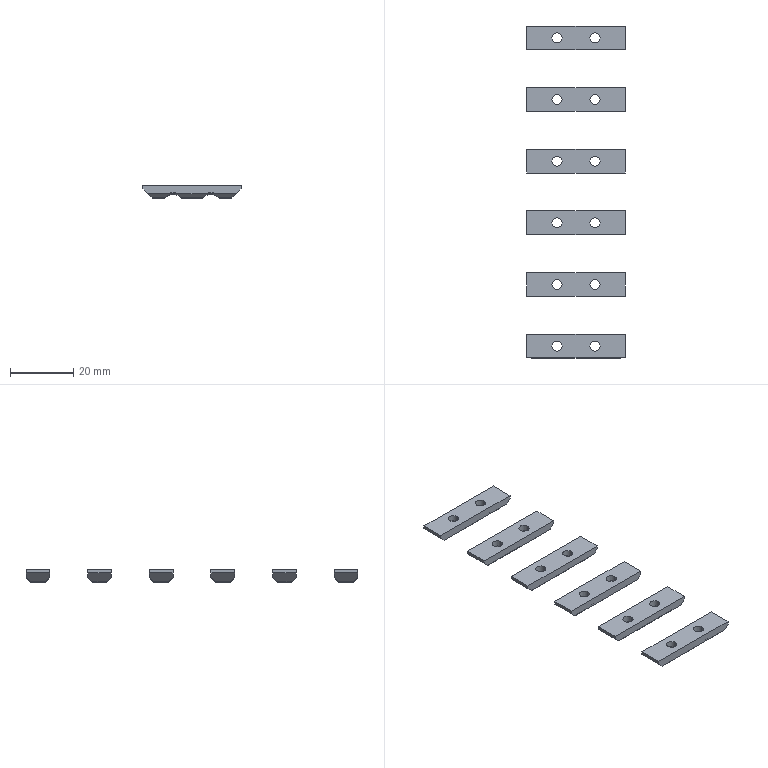NC program | NX | posted with a generic post | part box 31 x 105 x 4 mm
Lines 1425 to 2602 of 12738:
(ZLEVEL_PROFILE , TOOL : D4R0.5)
N2824 T16 M6
N2826 G54
N2828 G17 G0 G90 X52.171 Y-15.03 S9500 M3
N2830 G43 Z30. H16
N2832 Z2.9
N2834 G94 G1 Z-0.1 F2500.
N2836 X51.869 Y-14.507
N2838 G3 X51.522 Y-14.307 R0.4
N2840 G1 X46.185
N2842 X45.994 Y-14.306
N2844 X45.89 Y-14.394 Z-0.187
N2846 X51.516 Y-14.395
N2848 X51.61 Y-14.391
N2850 X51.68 Y-14.461 Z-0.258
N2852 X51.516 Y-14.465
N2854 X45.904
N2856 X45.82 Y-14.461
N2858 X45.749 Y-14.532 Z-0.329
N2860 X46.318 Y-14.536
N2862 X51.235
N2864 X51.751 Y-14.534
N2866 X51.822 Y-14.605 Z-0.4
N2868 X51.797 Y-14.607
N2870 X46.247
N2872 X45.678 Y-14.605
N2874 X45.607 Y-14.676 Z-0.47
N2876 X46.176 Y-14.677
N2878 X51.797
N2880 X51.893 Y-14.674
N2882 X51.963 Y-14.744 Z-0.541
N2884 X51.395 Y-14.748
N2886 X45.624
N2888 X45.537 Y-14.744
N2890 X45.466 Y-14.815 Z-0.612
N2892 X46.035 Y-14.819
N2894 X51.465
N2896 X52.034 Y-14.817
N2898 X52.105 Y-14.888 Z-0.682
N2900 X52.077 Y-14.89
N2902 X45.964
N2904 X45.395 Y-14.889
N2906 X45.325 Y-14.959 Z-0.753
N2908 X45.893 Y-14.96
N2910 X52.077
N2912 X52.175 Y-14.957
N2914 X52.246 Y-15.027 Z-0.824
N2916 X51.677 Y-15.031
N2918 X45.343
N2920 X45.254 Y-15.027
N2922 X45.184 Y-15.098 Z-0.895
N2924 X45.752 Y-15.102
N2926 X51.748
N2928 X52.316 Y-15.1
N2930 X52.387 Y-15.171 Z-0.965
N2932 X52.358 Y-15.172
N2934 X45.681
N2936 X45.113
N2938 X45.043 Y-15.242 Z-1.036
N2940 X45.063 Y-15.243
N2942 X52.358
N2944 X52.457 Y-15.239
N2946 X52.528 Y-15.31 Z-1.107
N2948 X51.96 Y-15.314
N2950 X45.063
N2952 X44.972 Y-15.31
N2954 X44.902 Y-15.381 Z-1.177
N2956 X45.469 Y-15.385
N2958 X52.031
N2960 X52.598 Y-15.383
N2962 X52.668 Y-15.454 Z-1.248
N2964 X52.102 Y-15.455
N2966 X45.398
N2968 X44.831
N2970 X44.761 Y-15.525 Z-1.319
N2972 X44.782 Y-15.526
N2974 X52.638
N2976 X52.739 Y-15.522
N2978 X52.809 Y-15.593 Z-1.39
N2980 X52.243 Y-15.597
N2982 X44.782
N2984 X44.691 Y-15.592
N2986 X44.621 Y-15.664 Z-1.46
N2988 X45.186 Y-15.667
N2990 X52.314
N2992 X52.88 Y-15.665
N2994 X52.944 Y-15.737 Z-1.531
N2996 X52.385 Y-15.738
N2998 X45.115
N3000 X44.556
N3002 X44.554 Y-15.773 Z-1.566
N3004 X44.551 Y-15.808 Z-1.602
N3006 X45.045 Y-15.809
N3008 X52.919
N3010 X52.949 Y-15.807
N3012 X52.951 Y-15.844 Z-1.637
N3014 X52.954 Y-15.878 Z-1.672
N3016 X52.919 Y-15.88
N3018 X45.
N3020 X44.546 Y-15.879
N3022 X44.544 Y-15.915 Z-1.708
N3024 X44.541 Y-15.95 Z-1.743
N3026 X45.
N3028 X52.919
N3030 X52.959 Y-15.948
N3032 X52.961 Y-15.986 Z-1.778
N3034 X52.963 Y-16.019 Z-1.814
N3036 X52.919 Y-16.021
N3038 X45.
N3040 X44.537
N3042 X44.536 Y-16.056 Z-1.849
N3044 Y-16.091 Z-1.885
N3046 X45. Y-16.092
N3048 X52.919
N3050 X52.964 Y-16.089
N3052 Y-16.127 Z-1.92
N3054 Y-16.16 Z-1.955
N3056 X52.919 Y-16.162
N3058 X45.
N3060 X44.536
N3062 X44.535 Y-16.198 Z-1.991
N3064 Y-16.233 Z-2.026
N3066 X45.
N3068 X52.919
N3070 X52.965 Y-16.231
N3072 Y-16.268 Z-2.061
N3074 Y-16.301 Z-2.097
N3076 X52.919 Y-16.304
N3078 X45.
N3080 X44.535
N3082 X44.534 Y-16.339 Z-2.132
N3084 Y-16.374 Z-2.167
N3086 X45.
N3088 X52.5
N3090 X52.966 Y-16.372
N3092 Y-16.41 Z-2.203
N3094 Y-16.443 Z-2.238
N3096 X52.919 Y-16.445
N3098 X45.
N3100 X44.534
N3102 X44.533 Y-16.481 Z-2.273
N3104 Y-16.516 Z-2.309
N3106 X45.
N3108 X52.919
N3110 X52.967 Y-16.513
N3112 Y-16.551 Z-2.344
N3114 Y-16.584 Z-2.38
N3116 X52.919 Y-16.587
N3118 X45.
N3120 X44.533 Y-16.586
N3122 Y-16.622 Z-2.415
N3124 X44.532 Y-16.657 Z-2.45
N3126 X45.
N3128 X52.919
N3130 X52.967 Y-16.655
N3132 X52.968 Y-16.693 Z-2.486
N3134 Y-16.726 Z-2.521
N3136 X52.919 Y-16.728
N3138 X45.
N3140 X44.532
N3142 Y-16.763 Z-2.556
N3144 Y-16.799 Z-2.592
N3146 X45.
N3148 X52.919
N3150 X52.968 Y-16.796
N3152 Y-16.834 Z-2.627
N3154 Y-16.867 Z-2.662
N3156 X52.919 Y-16.869
N3158 X45.
N3160 X44.531
N3162 Y-16.905 Z-2.698
N3164 Y-16.94 Z-2.733
N3166 X45.
N3168 X52.5
N3170 X52.969 Y-16.938
N3172 Y-16.976 Z-2.768
N3174 Y-17.008 Z-2.804
N3176 X52.919 Y-17.011
N3178 X45.
N3180 X44.531
N3182 Y-17.046 Z-2.839
N3184 Y-17.081 Z-2.874
N3186 X45. Y-17.082
N3188 X52.919
N3190 X52.969 Y-17.079
N3192 Y-17.117 Z-2.91
N3194 X52.97 Y-17.15 Z-2.945
N3196 X52.919 Y-17.152
N3198 X45.
N3200 X44.53
N3202 Y-17.188 Z-2.981
N3204 Y-17.223 Z-3.016
N3206 X45.
N3208 X52.919
N3210 X52.97 Y-17.22
N3212 Y-17.258 Z-3.051
N3214 Y-17.291 Z-3.087
N3216 X52.919 Y-17.294
N3218 X45.
N3220 X44.53
N3222 Y-17.329 Z-3.122
N3224 X44.529 Y-17.364 Z-3.157
N3226 X52.919
N3228 X52.97 Y-17.362
N3230 X52.971 Y-17.4 Z-3.193
N3232 Y-17.433 Z-3.228
N3234 X44.529 Y-17.435
N3236 Y-17.469 Z-3.262
N3238 Y-17.503 Z-3.296
N3240 X52.919
N3242 X52.971 Y-17.501
N3244 Y-17.537 Z-3.33
N3246 Y-17.568 Z-3.364
N3248 X52.919 Y-17.571
N3250 X44.529
N3252 X44.528 Y-17.605 Z-3.398
N3254 Y-17.639 Z-3.432
N3256 X52.919
N3258 X52.971 Y-17.636
N3260 G2 X53.327 Y-17.819 R0.4
N3262 G1 X53.666 Y-18.343
N3264 Z-0.432
N3266 G0 Z30.
N3268 X32.653 Y-15.036
N3270 Z2.9
N3272 G1 Z-0.1
N3274 X32.348 Y-14.506
N3276 G3 X32.001 Y-14.306 R0.4
N3278 G1 X26.499
N3280 X26.39 Y-14.392 Z-0.187
N3282 X26.429 Y-14.395
N3284 X32.071
N3286 X32.11 Y-14.392
N3288 X32.18 Y-14.461 Z-0.258
N3290 X32.071 Y-14.465
N3292 X26.429
N3294 X26.32 Y-14.461
N3296 X26.249 Y-14.532 Z-0.329
N3298 X26.711 Y-14.536
N3300 X31.789
N3302 X32.251 Y-14.532
N3304 X32.322 Y-14.606 Z-0.4
N3306 X31.753 Y-14.607
N3308 X26.747
N3310 X26.178 Y-14.606
N3312 X26.108 Y-14.675 Z-0.47
N3314 X26.147 Y-14.677
N3316 X32.353
N3318 X32.392 Y-14.675
N3320 X32.463 Y-14.744 Z-0.541
N3322 X32.353 Y-14.748
N3324 X26.147
N3326 X26.037 Y-14.744
N3328 X25.966 Y-14.815 Z-0.612
N3330 X26.429 Y-14.819
N3332 X32.071
N3334 X32.534 Y-14.815
N3336 X32.605 Y-14.889 Z-0.682
N3338 X32.036 Y-14.89
N3340 X26.464
N3342 X25.895 Y-14.889
N3344 X25.825 Y-14.958 Z-0.753
N3346 X25.865 Y-14.96
N3348 X32.635
N3350 X32.675 Y-14.958
N3352 X32.746 Y-15.026 Z-0.824
N3354 X32.635 Y-15.031
N3356 X25.865
N3358 X25.754 Y-15.026
N3360 X25.684 Y-15.098 Z-0.895
N3362 X26.147 Y-15.102
N3364 X32.353
N3366 X32.816 Y-15.098
N3368 X32.887 Y-15.172 Z-0.965
N3370 X32.319
N3372 X26.181
N3374 X25.613
N3376 X25.543 Y-15.241 Z-1.036
N3378 X25.583 Y-15.243
N3380 X32.917
N3382 X32.957 Y-15.241
N3384 X33.027 Y-15.309 Z-1.107
N3386 X32.917 Y-15.314
N3388 X25.583
N3390 X25.473 Y-15.309
N3392 X25.402 Y-15.381 Z-1.177
N3394 X25.865 Y-15.385
N3396 X32.635
N3398 X33.098 Y-15.381
N3400 X33.168 Y-15.455 Z-1.248
N3402 X32.602
N3404 X25.898
N3406 X25.332
N3408 X25.261 Y-15.523 Z-1.319
N3410 X25.301 Y-15.526
N3412 X33.199
N3414 X33.239 Y-15.523
N3416 X33.309 Y-15.592 Z-1.39
N3418 X33.199 Y-15.597
N3420 X25.301
N3422 X25.191 Y-15.592
N3424 X25.12 Y-15.664 Z-1.46
N3426 X25.686 Y-15.667
N3428 X32.814
N3430 X33.38 Y-15.664
N3432 X33.444 Y-15.738 Z-1.531
N3434 X32.885
N3436 X25.615
N3438 X25.056
N3440 X25.054 Y-15.773 Z-1.566
N3442 X25.051 Y-15.809 Z-1.602
N3444 X25.545
N3446 X32.955
N3448 X33.449
N3450 X33.451 Y-15.844 Z-1.637
N3452 X33.454 Y-15.879 Z-1.672
N3454 X33. Y-15.88
N3456 X25.5
N3458 X25.046 Y-15.879
N3460 X25.043 Y-15.915 Z-1.708
N3462 X25.041 Y-15.95 Z-1.743
N3464 X25.5
N3466 X33.
N3468 X33.459
N3470 X33.461 Y-15.986 Z-1.778
N3472 X33.463 Y-16.021 Z-1.814
N3474 X33.
N3476 X25.5
N3478 X25.037
N3480 X25.036 Y-16.056 Z-1.849
N3482 Y-16.092 Z-1.885
N3484 X25.5
N3486 X33.
N3488 X33.464
N3490 Y-16.127 Z-1.92
N3492 Y-16.162 Z-1.955
N3494 X33.
N3496 X25.5
N3498 X25.036
N3500 X25.035 Y-16.198 Z-1.991
N3502 Y-16.233 Z-2.026
N3504 X25.5
N3506 X33.
N3508 X33.465
N3510 Y-16.268 Z-2.061
N3512 Y-16.304 Z-2.097
N3514 X33.
N3516 X25.5
N3518 X25.035
N3520 X25.034 Y-16.339 Z-2.132
N3522 Y-16.374 Z-2.167
N3524 X25.5
N3526 X33.
N3528 X33.466
N3530 Y-16.41 Z-2.203
N3532 Y-16.445 Z-2.238
N3534 X33.
N3536 X25.5
N3538 X25.034
N3540 X25.033 Y-16.481 Z-2.273
N3542 Y-16.516 Z-2.309
N3544 X25.5
N3546 X33.
N3548 X33.467
N3550 Y-16.551 Z-2.344
N3552 Y-16.587 Z-2.38
N3554 X33.
N3556 X25.5
N3558 X25.033
N3560 Y-16.622 Z-2.415
N3562 X25.032 Y-16.657 Z-2.45
N3564 X25.5
N3566 X33.
N3568 X33.468
N3570 Y-16.693 Z-2.486
N3572 Y-16.728 Z-2.521
N3574 X33.
N3576 X25.5
N3578 X25.032
N3580 Y-16.763 Z-2.556
N3582 Y-16.799 Z-2.592
N3584 X25.5
N3586 X33.
N3588 X33.468
N3590 Y-16.834 Z-2.627
N3592 X33.469 Y-16.869 Z-2.662
N3594 X33.
N3596 X25.5
N3598 X25.031
N3600 Y-16.905 Z-2.698
N3602 Y-16.94 Z-2.733
N3604 X25.5
N3606 X33.
N3608 X33.469
N3610 Y-16.976 Z-2.768
N3612 Y-17.011 Z-2.804
N3614 X33.
N3616 X25.5
N3618 X25.031
N3620 Y-17.046 Z-2.839
N3622 Y-17.082 Z-2.874
N3624 X25.5
N3626 X33.
N3628 X33.469
N3630 X33.47 Y-17.117 Z-2.91
N3632 Y-17.152 Z-2.945
N3634 X33.
N3636 X25.5
N3638 X25.03
N3640 Y-17.188 Z-2.981
N3642 Y-17.223 Z-3.016
N3644 X25.5
N3646 X33.
N3648 X33.47
N3650 Y-17.258 Z-3.051
N3652 Y-17.294 Z-3.087
N3654 X33.
N3656 X25.5
N3658 X25.03
N3660 Y-17.329 Z-3.122
N3662 X25.029 Y-17.364 Z-3.157
N3664 X33.471
N3666 Y-17.4 Z-3.193
N3668 Y-17.435 Z-3.228
N3670 X25.029
N3672 Y-17.469 Z-3.262
N3674 Y-17.503 Z-3.296
N3676 X33.471
N3678 Y-17.537 Z-3.33
N3680 Y-17.571 Z-3.364
N3682 X25.029
N3684 X25.028 Y-17.605 Z-3.398
N3686 Y-17.639 Z-3.432
N3688 X33.472
N3690 G2 X33.818 Y-17.839 R0.4
N3692 G1 X34.117 Y-18.357
N3694 Z-0.432
N3696 G0 Z30.
N3698 X13.153 Y-15.036
N3700 Z2.9
N3702 G1 Z-0.1
N3704 X12.848 Y-14.506
N3706 G3 X12.501 Y-14.306 R0.4
N3708 G1 X6.999
N3710 X6.89 Y-14.392 Z-0.187
N3712 X6.929 Y-14.395
N3714 X12.571
N3716 X12.61 Y-14.392
N3718 X12.68 Y-14.461 Z-0.258
N3720 X12.571 Y-14.465
N3722 X6.929
N3724 X6.82 Y-14.461
N3726 X6.749 Y-14.532 Z-0.329
N3728 X7.211 Y-14.536
N3730 X12.289
N3732 X12.751 Y-14.532
N3734 X12.822 Y-14.606 Z-0.4
N3736 X12.253 Y-14.607
N3738 X7.247
N3740 X6.678 Y-14.606
N3742 X6.608 Y-14.675 Z-0.47
N3744 X6.647 Y-14.677
N3746 X12.853
N3748 X12.892 Y-14.675
N3750 X12.963 Y-14.744 Z-0.541
N3752 X12.853 Y-14.748
N3754 X6.647
N3756 X6.537 Y-14.744
N3758 X6.466 Y-14.815 Z-0.612
N3760 X6.929 Y-14.819
N3762 X12.571
N3764 X13.034 Y-14.815
N3766 X13.105 Y-14.889 Z-0.682
N3768 X12.536 Y-14.89
N3770 X6.964
N3772 X6.395 Y-14.889
N3774 X6.325 Y-14.958 Z-0.753
N3776 X6.365 Y-14.96
N3778 X13.135
N3780 X13.175 Y-14.958
N3782 X13.246 Y-15.026 Z-0.824
N3784 X13.135 Y-15.031
N3786 X6.365
N3788 X6.254 Y-15.026
N3790 X6.184 Y-15.098 Z-0.895
N3792 X6.647 Y-15.102
N3794 X12.853
N3796 X13.316 Y-15.098
N3798 X13.387 Y-15.172 Z-0.965
N3800 X12.819
N3802 X6.681
N3804 X6.113
N3806 X6.043 Y-15.241 Z-1.036
N3808 X6.083 Y-15.243
N3810 X13.417
N3812 X13.457 Y-15.241
N3814 X13.527 Y-15.309 Z-1.107
N3816 X13.417 Y-15.314
N3818 X6.083
N3820 X5.973 Y-15.309
N3822 X5.902 Y-15.381 Z-1.177
N3824 X6.365 Y-15.385
N3826 X13.135
N3828 X13.598 Y-15.381
N3830 X13.668 Y-15.455 Z-1.248
N3832 X13.102
N3834 X6.398
N3836 X5.832
N3838 X5.761 Y-15.523 Z-1.319
N3840 X5.801 Y-15.526
N3842 X13.699
N3844 X13.739 Y-15.523
N3846 X13.809 Y-15.592 Z-1.39
N3848 X13.699 Y-15.597
N3850 X5.801
N3852 X5.691 Y-15.592
N3854 X5.62 Y-15.664 Z-1.46
N3856 X6.186 Y-15.667
N3858 X13.314
N3860 X13.88 Y-15.664
N3862 X13.944 Y-15.738 Z-1.531
N3864 X13.385
N3866 X6.115
N3868 X5.556
N3870 X5.554 Y-15.773 Z-1.566
N3872 X5.551 Y-15.809 Z-1.602
N3874 X6.045
N3876 X13.455
N3878 X13.949
N3880 X13.951 Y-15.844 Z-1.637
N3882 X13.954 Y-15.879 Z-1.672
N3884 X13.5 Y-15.88
N3886 X6.
N3888 X5.546 Y-15.879
N3890 X5.543 Y-15.915 Z-1.708
N3892 X5.541 Y-15.95 Z-1.743
N3894 X6.
N3896 X13.5
N3898 X13.959
N3900 X13.961 Y-15.986 Z-1.778
N3902 X13.963 Y-16.021 Z-1.814
N3904 X13.5
N3906 X6.
N3908 X5.537
N3910 X5.536 Y-16.056 Z-1.849
N3912 Y-16.092 Z-1.885
N3914 X6.
N3916 X13.5
N3918 X13.964
N3920 Y-16.127 Z-1.92
N3922 Y-16.162 Z-1.955
N3924 X13.5
N3926 X6.
N3928 X5.536
N3930 X5.535 Y-16.198 Z-1.991
N3932 Y-16.233 Z-2.026
N3934 X6.
N3936 X13.5
N3938 X13.965
N3940 Y-16.268 Z-2.061
N3942 Y-16.304 Z-2.097
N3944 X13.5
N3946 X6.
N3948 X5.535
N3950 X5.534 Y-16.339 Z-2.132
N3952 Y-16.374 Z-2.167
N3954 X6.
N3956 X13.5
N3958 X13.966
N3960 Y-16.41 Z-2.203
N3962 Y-16.445 Z-2.238
N3964 X13.5
N3966 X6.
N3968 X5.534
N3970 X5.533 Y-16.481 Z-2.273
N3972 Y-16.516 Z-2.309
N3974 X6.
N3976 X13.5
N3978 X13.967
N3980 Y-16.551 Z-2.344
N3982 Y-16.587 Z-2.38
N3984 X13.5
N3986 X6.
N3988 X5.533
N3990 Y-16.622 Z-2.415
N3992 X5.532 Y-16.657 Z-2.45
N3994 X6.
N3996 X13.5
N3998 X13.968
N4000 Y-16.693 Z-2.486
N4002 Y-16.728 Z-2.521
N4004 X13.5
N4006 X6.
N4008 X5.532
N4010 Y-16.763 Z-2.556
N4012 Y-16.799 Z-2.592
N4014 X6.
N4016 X13.5
N4018 X13.968
N4020 Y-16.834 Z-2.627
N4022 X13.969 Y-16.869 Z-2.662
N4024 X13.5
N4026 X6.
N4028 X5.531
N4030 Y-16.905 Z-2.698
N4032 Y-16.94 Z-2.733
N4034 X6.
N4036 X13.5
N4038 X13.969
N4040 Y-16.976 Z-2.768
N4042 Y-17.011 Z-2.804
N4044 X13.5
N4046 X6.
N4048 X5.531
N4050 Y-17.046 Z-2.839
N4052 Y-17.082 Z-2.874
N4054 X6.
N4056 X13.5
N4058 X13.969
N4060 X13.97 Y-17.117 Z-2.91
N4062 Y-17.152 Z-2.945
N4064 X13.5
N4066 X6.
N4068 X5.53
N4070 Y-17.188 Z-2.981
N4072 Y-17.223 Z-3.016
N4074 X6.
N4076 X13.5
N4078 X13.97
N4080 Y-17.258 Z-3.051
N4082 Y-17.294 Z-3.087
N4084 X13.5
N4086 X6.
N4088 X5.53
N4090 Y-17.329 Z-3.122
N4092 X5.529 Y-17.364 Z-3.157
N4094 X13.971
N4096 Y-17.4 Z-3.193
N4098 Y-17.435 Z-3.228
N4100 X5.529
N4102 Y-17.469 Z-3.262
N4104 Y-17.503 Z-3.296
N4106 X13.971
N4108 Y-17.537 Z-3.33
N4110 Y-17.571 Z-3.364
N4112 X5.529
N4114 X5.528 Y-17.605 Z-3.398
N4116 Y-17.639 Z-3.432
N4118 X13.972
N4120 G2 X14.318 Y-17.839 R0.4
N4122 G1 X14.617 Y-18.357
N4124 Z-0.432
N4126 G0 Z30.
N4128 X-6.347 Y-15.036
N4130 Z2.9
N4132 G1 Z-0.1
N4134 X-6.652 Y-14.506
N4136 G3 X-6.999 Y-14.306 R0.4
N4138 G1 X-12.501
N4140 X-12.61 Y-14.392 Z-0.187
N4142 X-12.571 Y-14.395
N4144 X-6.929
N4146 X-6.89 Y-14.392
N4148 X-6.82 Y-14.461 Z-0.258
N4150 X-6.929 Y-14.465
N4152 X-12.571
N4154 X-12.68 Y-14.461
N4156 X-12.751 Y-14.532 Z-0.329
N4158 X-12.289 Y-14.536
N4160 X-7.211
N4162 X-6.749 Y-14.532
N4164 X-6.678 Y-14.606 Z-0.4
N4166 X-7.247 Y-14.607
N4168 X-12.253
N4170 X-12.822 Y-14.606
N4172 X-12.892 Y-14.675 Z-0.47
N4174 X-12.853 Y-14.677
N4176 X-6.647
N4178 X-6.608 Y-14.675
N4180 X-6.537 Y-14.744 Z-0.541
N4182 X-6.647 Y-14.748
N4184 X-12.853
N4186 X-12.963 Y-14.744
N4188 X-13.034 Y-14.815 Z-0.612
N4190 X-12.571 Y-14.819
N4192 X-6.929
N4194 X-6.466 Y-14.815
N4196 X-6.395 Y-14.889 Z-0.682
N4198 X-6.964 Y-14.89
N4200 X-12.536
N4202 X-13.105 Y-14.889
N4204 X-13.175 Y-14.958 Z-0.753
N4206 X-13.135 Y-14.96
N4208 X-6.365
N4210 X-6.325 Y-14.958
N4212 X-6.254 Y-15.026 Z-0.824
N4214 X-6.365 Y-15.031
N4216 X-13.135
N4218 X-13.246 Y-15.026
N4220 X-13.316 Y-15.098 Z-0.895
N4222 X-12.853 Y-15.102
N4224 X-6.647
N4226 X-6.184 Y-15.098
N4228 X-6.113 Y-15.172 Z-0.965
N4230 X-6.681
N4232 X-12.819
N4234 X-13.387
N4236 X-13.457 Y-15.241 Z-1.036
N4238 X-13.417 Y-15.243
N4240 X-6.083
N4242 X-6.043 Y-15.241
N4244 X-5.973 Y-15.309 Z-1.107
N4246 X-6.083 Y-15.314
N4248 X-13.417
N4250 X-13.527 Y-15.309
N4252 X-13.598 Y-15.381 Z-1.177
N4254 X-13.135 Y-15.385
N4256 X-6.365
N4258 X-5.902 Y-15.381
N4260 X-5.832 Y-15.455 Z-1.248
N4262 X-6.398
N4264 X-13.102
N4266 X-13.668
N4268 X-13.739 Y-15.523 Z-1.319
N4270 X-13.699 Y-15.526
N4272 X-5.801
N4274 X-5.761 Y-15.523
N4276 X-5.691 Y-15.592 Z-1.39
N4278 X-5.801 Y-15.597
N4280 X-13.699
N4282 X-13.809 Y-15.592
N4284 X-13.88 Y-15.664 Z-1.46
N4286 X-13.314 Y-15.667
N4288 X-6.186
N4290 X-5.62 Y-15.664
N4292 X-5.556 Y-15.738 Z-1.531
N4294 X-6.115
N4296 X-13.385
N4298 X-13.944
N4300 X-13.946 Y-15.773 Z-1.566
N4302 X-13.949 Y-15.809 Z-1.602
N4304 X-13.455
N4306 X-6.045
N4308 X-5.551
N4310 X-5.549 Y-15.844 Z-1.637
N4312 X-5.546 Y-15.879 Z-1.672
N4314 X-6. Y-15.88
N4316 X-13.5
N4318 X-13.954 Y-15.879
N4320 X-13.957 Y-15.915 Z-1.708
N4322 X-13.959 Y-15.95 Z-1.743
N4324 X-13.5
N4326 X-6.
N4328 X-5.541
N4330 X-5.539 Y-15.986 Z-1.778
N4332 X-5.537 Y-16.021 Z-1.814
N4334 X-6.
N4336 X-13.5
N4338 X-13.963
N4340 X-13.964 Y-16.056 Z-1.849
N4342 Y-16.092 Z-1.885
N4344 X-13.5
N4346 X-6.
N4348 X-5.536
N4350 Y-16.127 Z-1.92
N4352 Y-16.162 Z-1.955
N4354 X-6.
N4356 X-13.5
N4358 X-13.964
N4360 X-13.965 Y-16.198 Z-1.991
N4362 Y-16.233 Z-2.026
N4364 X-13.5
N4366 X-6.
N4368 X-5.535
N4370 Y-16.268 Z-2.061
N4372 Y-16.304 Z-2.097
N4374 X-6.
N4376 X-13.5
N4378 X-13.965
N4380 X-13.966 Y-16.339 Z-2.132
N4382 Y-16.374 Z-2.167
N4384 X-13.5
N4386 X-6.
N4388 X-5.534
N4390 Y-16.41 Z-2.203
N4392 Y-16.445 Z-2.238
N4394 X-6.
N4396 X-13.5
N4398 X-13.966
N4400 X-13.967 Y-16.481 Z-2.273
N4402 Y-16.516 Z-2.309
N4404 X-13.5
N4406 X-6.
N4408 X-5.533
N4410 Y-16.551 Z-2.344
N4412 Y-16.587 Z-2.38
N4414 X-6.
N4416 X-13.5
N4418 X-13.967
N4420 Y-16.622 Z-2.415
N4422 X-13.968 Y-16.657 Z-2.45
N4424 X-13.5
N4426 X-6.
N4428 X-5.532
N4430 Y-16.693 Z-2.486
N4432 Y-16.728 Z-2.521
N4434 X-6.
N4436 X-13.5
N4438 X-13.968
N4440 Y-16.763 Z-2.556
N4442 Y-16.799 Z-2.592
N4444 X-13.5
N4446 X-6.
N4448 X-5.532
N4450 Y-16.834 Z-2.627
N4452 X-5.531 Y-16.869 Z-2.662
N4454 X-6.
N4456 X-13.5
N4458 X-13.969
N4460 Y-16.905 Z-2.698
N4462 Y-16.94 Z-2.733
N4464 X-13.5
N4466 X-6.
N4468 X-5.531
N4470 Y-16.976 Z-2.768
N4472 Y-17.011 Z-2.804
N4474 X-6.
N4476 X-13.5
N4478 X-13.969
N4480 Y-17.046 Z-2.839
N4482 Y-17.082 Z-2.874
N4484 X-13.5
N4486 X-6.
N4488 X-5.531
N4490 X-5.53 Y-17.117 Z-2.91
N4492 Y-17.152 Z-2.945
N4494 X-6.
N4496 X-13.5
N4498 X-13.97
N4500 Y-17.188 Z-2.981
N4502 Y-17.223 Z-3.016
N4504 X-13.5
N4506 X-6.
N4508 X-5.53
N4510 Y-17.258 Z-3.051
N4512 Y-17.294 Z-3.087
N4514 X-6.
N4516 X-13.5
N4518 X-13.97
N4520 Y-17.329 Z-3.122
N4522 X-13.971 Y-17.364 Z-3.157
N4524 X-5.529
N4526 Y-17.4 Z-3.193
N4528 Y-17.435 Z-3.228
N4530 X-13.971
N4532 Y-17.469 Z-3.262
N4534 Y-17.503 Z-3.296
N4536 X-5.529
N4538 Y-17.537 Z-3.33
N4540 Y-17.571 Z-3.364
N4542 X-13.971
N4544 X-13.972 Y-17.605 Z-3.398
N4546 Y-17.639 Z-3.432
N4548 X-5.528
N4550 G2 X-5.182 Y-17.839 R0.4
N4552 G1 X-4.883 Y-18.357
N4554 Z-0.432
N4556 G0 Z30.
N4558 X-25.847 Y-15.036
N4560 Z2.9
N4562 G1 Z-0.1
N4564 X-26.152 Y-14.506
N4566 G3 X-26.499 Y-14.306 R0.4
N4568 G1 X-32.001
N4570 X-32.11 Y-14.392 Z-0.187
N4572 X-32.071 Y-14.395
N4574 X-26.429
N4576 X-26.39 Y-14.392
N4578 X-26.32 Y-14.461 Z-0.258
N4580 X-26.429 Y-14.465
N4582 X-32.071
N4584 X-32.18 Y-14.461
N4586 X-32.251 Y-14.532 Z-0.329
N4588 X-31.789 Y-14.536
N4590 X-26.711
N4592 X-26.249 Y-14.532
N4594 X-26.178 Y-14.606 Z-0.4
N4596 X-26.747 Y-14.607
N4598 X-31.753
N4600 X-32.322 Y-14.606
N4602 X-32.392 Y-14.675 Z-0.47
N4604 X-32.353 Y-14.677
N4606 X-26.147
N4608 X-26.108 Y-14.675
N4610 X-26.037 Y-14.744 Z-0.541
N4612 X-26.147 Y-14.748
N4614 X-32.353
N4616 X-32.463 Y-14.744
N4618 X-32.534 Y-14.815 Z-0.612
N4620 X-32.071 Y-14.819
N4622 X-26.429
N4624 X-25.966 Y-14.815
N4626 X-25.895 Y-14.889 Z-0.682
N4628 X-26.464 Y-14.89
N4630 X-32.036
N4632 X-32.605 Y-14.889
N4634 X-32.675 Y-14.958 Z-0.753
N4636 X-32.635 Y-14.96
N4638 X-25.865
N4640 X-25.825 Y-14.958
N4642 X-25.754 Y-15.026 Z-0.824
N4644 X-25.865 Y-15.031
N4646 X-32.635
N4648 X-32.746 Y-15.026
N4650 X-32.816 Y-15.098 Z-0.895
N4652 X-32.353 Y-15.102
N4654 X-26.147
N4656 X-25.684 Y-15.098
N4658 X-25.613 Y-15.172 Z-0.965
N4660 X-26.181
N4662 X-32.319
N4664 X-32.887
N4666 X-32.957 Y-15.241 Z-1.036
N4668 X-32.917 Y-15.243
N4670 X-25.583
N4672 X-25.543 Y-15.241
N4674 X-25.473 Y-15.309 Z-1.107
N4676 X-25.583 Y-15.314
N4678 X-32.917
N4680 X-33.027 Y-15.309
N4682 X-33.098 Y-15.381 Z-1.177
N4684 X-32.635 Y-15.385
N4686 X-25.865
N4688 X-25.402 Y-15.381
N4690 X-25.332 Y-15.455 Z-1.248
N4692 X-25.898
N4694 X-32.602
N4696 X-33.168
N4698 X-33.239 Y-15.523 Z-1.319
N4700 X-33.199 Y-15.526
N4702 X-25.301
N4704 X-25.261 Y-15.523
N4706 X-25.191 Y-15.592 Z-1.39
N4708 X-25.301 Y-15.597
N4710 X-33.199
N4712 X-33.309 Y-15.592
N4714 X-33.38 Y-15.664 Z-1.46
N4716 X-32.814 Y-15.667
N4718 X-25.686
N4720 X-25.12 Y-15.664
N4722 X-25.056 Y-15.738 Z-1.531
N4724 X-25.615
N4726 X-32.885
N4728 X-33.444
N4730 X-33.446 Y-15.773 Z-1.566
N4732 X-33.449 Y-15.809 Z-1.602
N4734 X-32.955
N4736 X-25.545
N4738 X-25.051
N4740 X-25.049 Y-15.844 Z-1.637
N4742 X-25.046 Y-15.879 Z-1.672
N4744 X-25.5 Y-15.88
N4746 X-33.
N4748 X-33.454 Y-15.879
N4750 X-33.457 Y-15.915 Z-1.708
N4752 X-33.459 Y-15.95 Z-1.743
N4754 X-33.
N4756 X-25.5
N4758 X-25.041
N4760 X-25.039 Y-15.986 Z-1.778
N4762 X-25.037 Y-16.021 Z-1.814
N4764 X-25.5
N4766 X-33.
N4768 X-33.463
N4770 X-33.464 Y-16.056 Z-1.849
N4772 Y-16.092 Z-1.885
N4774 X-33.
N4776 X-25.5
N4778 X-25.036
N4780 Y-16.127 Z-1.92
N4782 Y-16.162 Z-1.955
N4784 X-25.5
N4786 X-33.
N4788 X-33.464
N4790 X-33.465 Y-16.198 Z-1.991
N4792 Y-16.233 Z-2.026
N4794 X-33.
N4796 X-25.5
N4798 X-25.035
N4800 Y-16.268 Z-2.061
N4802 Y-16.304 Z-2.097
N4804 X-25.5
N4806 X-33.
N4808 X-33.465
N4810 X-33.466 Y-16.339 Z-2.132
N4812 Y-16.374 Z-2.167
N4814 X-33.
N4816 X-25.5
N4818 X-25.034
N4820 Y-16.41 Z-2.203
N4822 Y-16.445 Z-2.238
N4824 X-25.5
N4826 X-33.
N4828 X-33.466
N4830 X-33.467 Y-16.481 Z-2.273
N4832 Y-16.516 Z-2.309
N4834 X-33.
N4836 X-25.5
N4838 X-25.033
N4840 Y-16.551 Z-2.344
N4842 Y-16.587 Z-2.38
N4844 X-25.5
N4846 X-33.
N4848 X-33.467
N4850 Y-16.622 Z-2.415
N4852 X-33.468 Y-16.657 Z-2.45
N4854 X-33.
N4856 X-25.5
N4858 X-25.032
N4860 Y-16.693 Z-2.486
N4862 Y-16.728 Z-2.521
N4864 X-25.5
N4866 X-33.
N4868 X-33.468
N4870 Y-16.763 Z-2.556
N4872 Y-16.799 Z-2.592
N4874 X-33.
N4876 X-25.5
N4878 X-25.032
N4880 Y-16.834 Z-2.627
N4882 X-25.031 Y-16.869 Z-2.662
N4884 X-25.5
N4886 X-33.
N4888 X-33.469
N4890 Y-16.905 Z-2.698
N4892 Y-16.94 Z-2.733
N4894 X-33.
N4896 X-25.5
N4898 X-25.031
N4900 Y-16.976 Z-2.768
N4902 Y-17.011 Z-2.804
N4904 X-25.5
N4906 X-33.
N4908 X-33.469
N4910 Y-17.046 Z-2.839
N4912 Y-17.082 Z-2.874
N4914 X-33.
N4916 X-25.5
N4918 X-25.031
N4920 X-25.03 Y-17.117 Z-2.91
N4922 Y-17.152 Z-2.945
N4924 X-25.5
N4926 X-33.
N4928 X-33.47
N4930 Y-17.188 Z-2.981
N4932 Y-17.223 Z-3.016
N4934 X-33.
N4936 X-25.5
N4938 X-25.03
N4940 Y-17.258 Z-3.051
N4942 Y-17.294 Z-3.087
N4944 X-25.5
N4946 X-33.
N4948 X-33.47
N4950 Y-17.329 Z-3.122
N4952 X-33.471 Y-17.364 Z-3.157
N4954 X-25.029
N4956 Y-17.4 Z-3.193
N4958 Y-17.435 Z-3.228
N4960 X-33.471
N4962 Y-17.469 Z-3.262
N4964 Y-17.503 Z-3.296
N4966 X-25.029
N4968 Y-17.537 Z-3.33
N4970 Y-17.571 Z-3.364
N4972 X-33.471
N4974 X-33.472 Y-17.605 Z-3.398
N4976 Y-17.639 Z-3.432
N4978 X-25.028
N4980 G2 X-24.682 Y-17.839 R0.4
N4982 G1 X-24.383 Y-18.357
N4984 Z-0.432
N4986 G0 Z30.
N4988 X-45.28 Y-15.02
N4990 Z2.9
N4992 G1 Z-0.1
N4994 X-45.669 Y-14.499
N4996 G3 X-46.036 Y-14.341 R0.4
N4998 G1 X-46.193 Y-14.35
N5000 X-51.235
N5002 X-51.383 Y-14.345
N5004 X-51.509 Y-14.34 Z-0.129
N5006 X-51.635 Y-14.334 Z-0.158
N5008 X-51.762 Y-14.338 Z-0.187
N5010 X-51.638 Y-14.339
N5012 X-51.511 Y-14.347
N5014 X-51.235 Y-14.35
N5016 X-46.185
N5018 X-45.885 Y-14.341
N5020 X-45.737 Y-14.336
N5022 X-45.703 Y-14.454 Z-0.258
N5024 X-46.343 Y-14.457
N5026 X-46.36 Y-14.461
N5028 X-51.148
N5030 X-51.165 Y-14.457
N5032 X-51.779 Y-14.456
N5034 X-51.788 Y-14.5 Z-0.294
N5036 X-51.796 Y-14.536 Z-0.329
N5038 X-51.182
N5040 X-46.318
N5042 X-46.299 Y-14.535
N5044 X-45.67 Y-14.533
N5046 X-45.636 Y-14.607 Z-0.4
N5048 X-46.247
N5050 X-51.797
N5052 X-51.861 Y-14.604
N5054 X-51.93 Y-14.674 Z-0.47
N5056 X-51.324 Y-14.677
N5058 X-45.624
N5060 X-45.57 Y-14.674
N5062 X-45.501 Y-14.744 Z-0.541
N5064 X-46.105 Y-14.748
N5066 X-51.395
N5068 X-51.999 Y-14.745
N5070 X-52.067 Y-14.818 Z-0.612
N5072 X-51.465 Y-14.819
N5074 X-46.035
N5076 X-45.433 Y-14.815
N5078 X-45.364 Y-14.889 Z-0.682
N5080 X-45.964 Y-14.89
N5082 X-51.536
N5084 X-52.136 Y-14.889
N5086 X-52.204 Y-14.957 Z-0.753
N5088 X-51.607 Y-14.96
N5090 X-45.343
N5092 X-45.296 Y-14.958
N5094 X-45.228 Y-15.027 Z-0.824
N5096 X-45.343 Y-15.031
N5098 X-51.677
N5100 X-52.272 Y-15.028
N5102 X-52.34 Y-15.101 Z-0.895
N5104 X-51.748 Y-15.102
N5106 X-45.752
N5108 X-45.16 Y-15.098
N5110 X-45.092 Y-15.172 Z-0.965
N5112 X-45.681
N5114 X-52.358
N5116 X-52.408 Y-15.171
N5118 X-52.476 Y-15.239 Z-1.036
N5120 X-51.89 Y-15.243
N5122 X-45.063
N5124 X-45.024 Y-15.241
N5126 X-44.956 Y-15.309 Z-1.107
N5128 X-45.063 Y-15.314
N5130 X-51.96
N5132 X-52.544 Y-15.31
N5134 X-52.611 Y-15.383 Z-1.177
N5136 X-52.031 Y-15.385
N5138 X-45.469
N5140 X-44.889 Y-15.381
N5142 X-44.821 Y-15.455 Z-1.248
N5144 X-45.398
N5146 X-52.638
N5148 X-52.679 Y-15.453
N5150 X-52.747 Y-15.522 Z-1.319
N5152 X-52.638 Y-15.526
N5154 X-44.782
N5156 X-44.753 Y-15.524
N5158 X-44.686 Y-15.592 Z-1.39
N5160 X-44.782 Y-15.597
N5162 X-52.243
N5164 X-52.814 Y-15.593
N5166 X-52.882 Y-15.665 Z-1.46
N5168 X-52.314 Y-15.667
N5170 X-45.186
N5172 X-44.618 Y-15.664